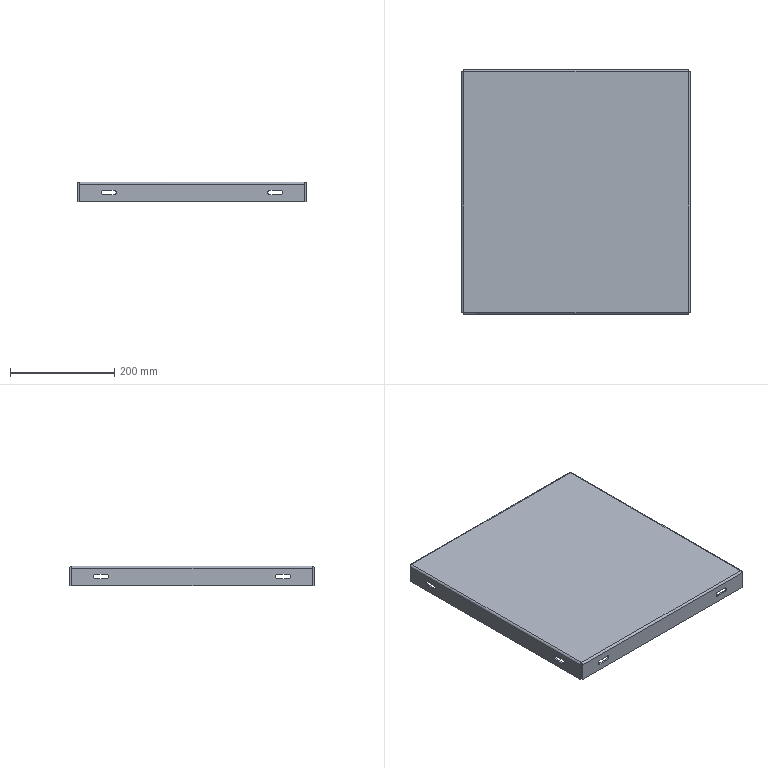Part | NX | features BREP 1 | 1 solid | 70 faces | box 439 x 469 x 38 mm | volume 793869 mm3 | plane 38 | cylinder 24 | spline 8 | commonest cylinder face diameters 8.5 x16 2 x4 8 x4